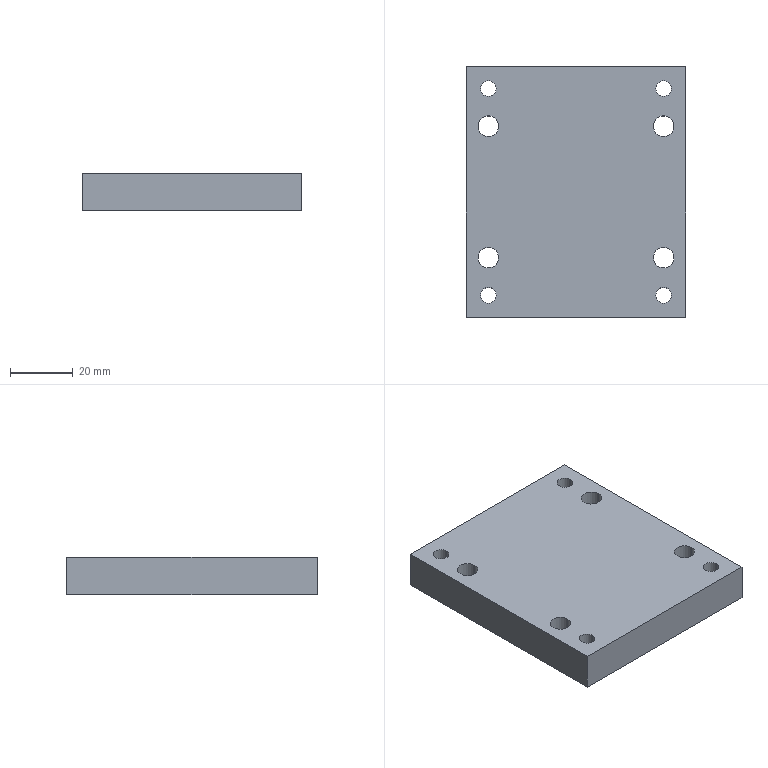Part | SolidWorks | features HoleWzd 2, Cut 1, Extrusion 1, LPattern 1 | 1 solid | 82 faces | box 70 x 80 x 12 mm | volume 59166 mm3 | cylinder 48 | plane 34 | commonest cylinder face diameters 5 x32 6.6 x8 11 x8